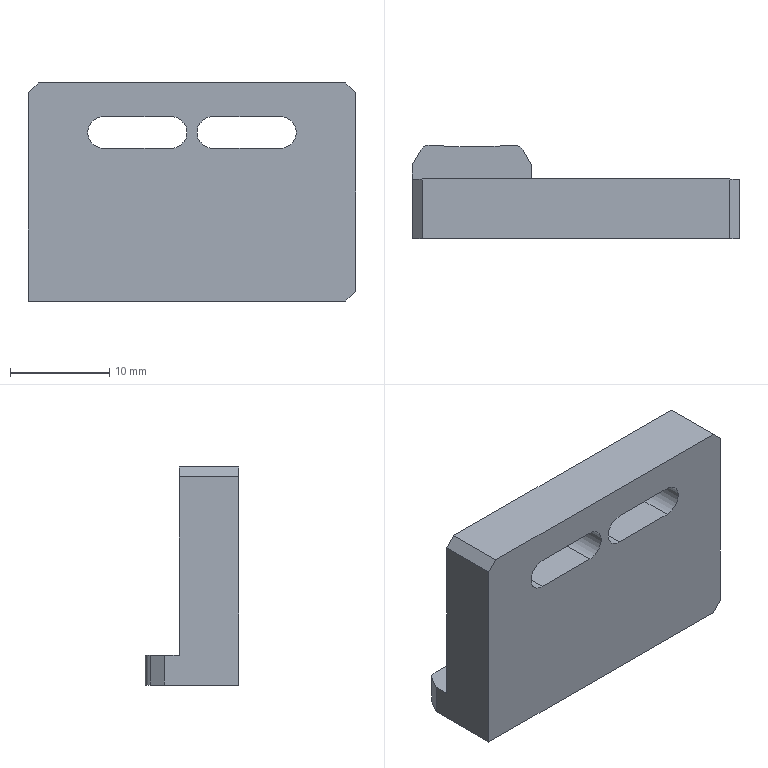Part | STEP file | secondary positioning block | 1 solid | 24 faces | box 33 x 9.454 x 22 mm | volume 4103 mm3 | plane 17 | cylinder 7 | commonest cylinder face diameters 3.2 x4 2 x2 88.5 x1